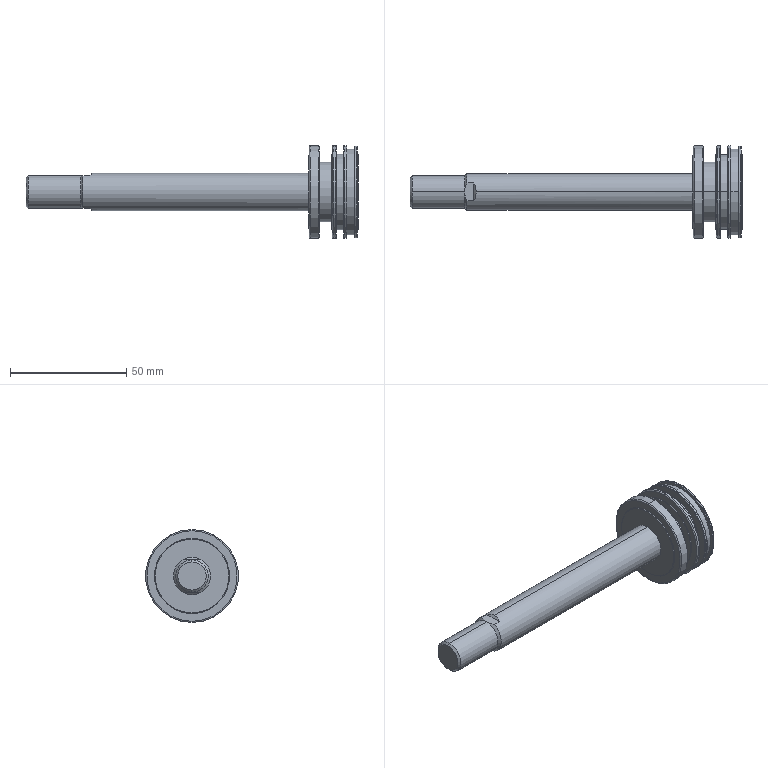Part | STEP file | ACQS_40x80_B_80r | 1 solid | 60 faces | box 143 x 40 x 40 mm | volume 43643 mm3 | cylinder 18 | plane 16 | torus 14 | cone 12 | commonest cylinder face diameters 40 x6 14 x2 16 x2 25.8 x2 32.4 x2 37 x2